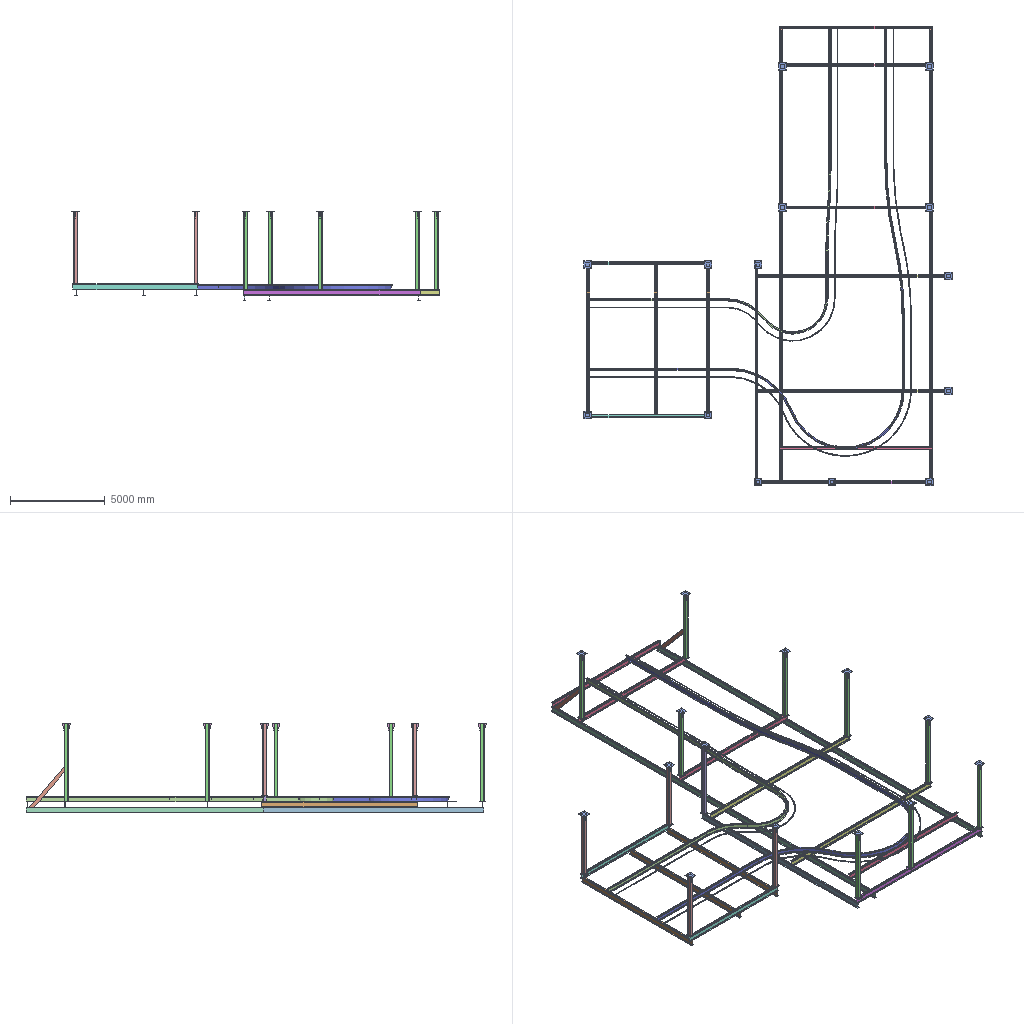Assembly | SolidWorks | 22 different items | 106 placed | box 19450 x 24300 x 4750 mm
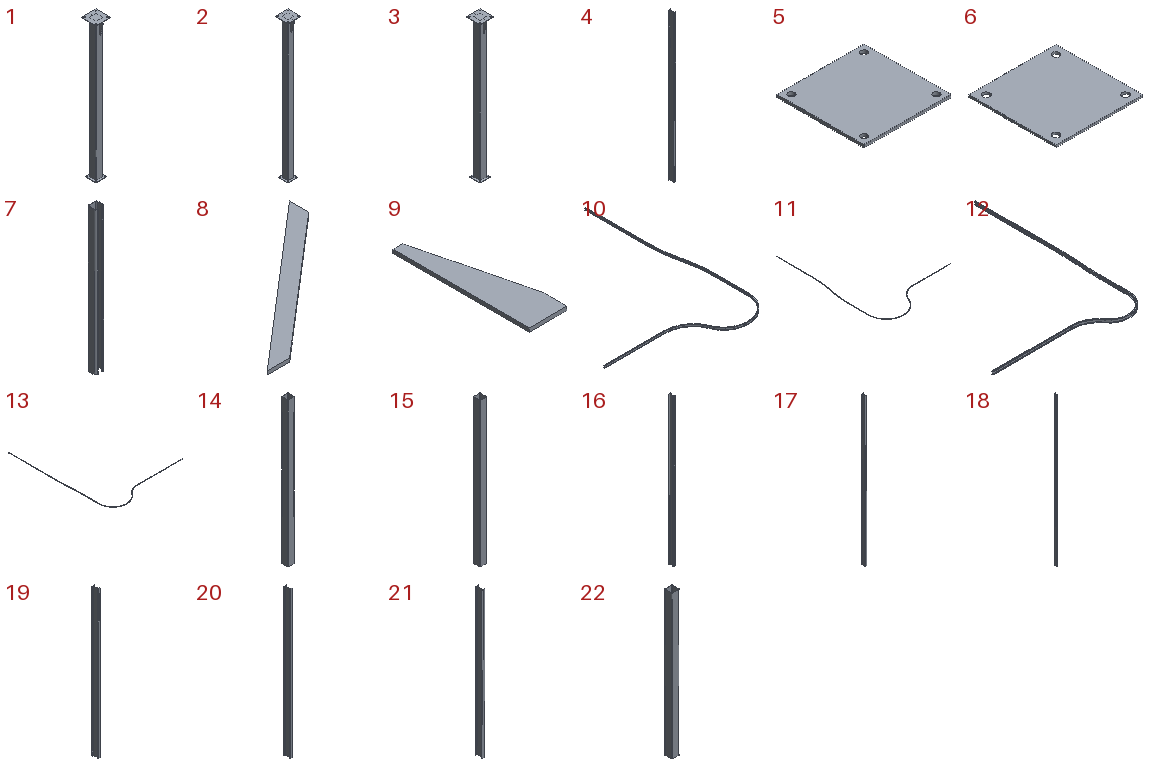Parts list (item | name | quantity | parent item | size | volume | features):
1 | (subassembly) | x4 | - | 400 x 400 x 3850 mm | 25640494 mm3 | -
2 | (subassembly) | x1 | - | 400 x 400 x 4450 mm | 29195042 mm3 | -
3 | (subassembly) | x9 | - | 400 x 400 x 4150 mm | 27417768 mm3 | -
4 | - | x1 | - | 150 x 300 x 9347 mm | 43725928 mm3 | features Extrusion 1
5 | - | x14 | in 1, 2, 3 | 300 x 300 x 10 mm | 884795 mm3 | features Extrusion 1
6 | - | x14 | in 1, 2, 3 | 400 x 400 x 10 mm | 1567830 mm3 | features Extrusion 1
7 | - | x1 | - | 32 x 30 x 500 mm | 85540 mm3 | features Extrusion 1
8 | - | x2 | - | 2174 x 1869 x 50 mm | 26646819 mm3 | features Extrusion 1
9 | - | x28 | in 1, 2, 3 | 100 x 360 x 10 mm | 249000 mm3 | features Extrusion 1
10 | - | x1 | - | 16778 x 22359 x 250 mm | 204415095 mm3 | features BaseBody 1
11 | - | x1 | - | 17149 x 22725 x 30 mm | 6973781 mm3 | features Sweep 1
12 | - | x1 | - | 12904 x 16279 x 250 mm | 148415394 mm3 | features BaseBody 1
13 | - | x1 | - | 13271 x 16645 x 30 mm | 5014402 mm3 | features Sweep 1
14 | - | x1 | in 2 | 200 x 200 x 4430 mm | 26244417 mm3 | features Extrusion 1
15 | - | x9 | in 3 | 200 x 200 x 4130 mm | 24467143 mm3 | features Extrusion 1
16 | - | x2 | - | 150 x 300 x 10347 mm | 48403999 mm3 | features Extrusion 1
17 | - | x1 | - | 150 x 300 x 11647 mm | 54485491 mm3 | features Extrusion 1
18 | - | x2 | - | 150 x 300 x 24174 mm | 113087685 mm3 | features Extrusion 1
19 | - | x3 | - | 150 x 300 x 8240 mm | 38547304 mm3 | features Extrusion 1
20 | - | x4 | - | 150 x 300 x 8060 mm | 37705251 mm3 | features Extrusion 1
21 | - | x2 | - | 150 x 300 x 6592 mm | 30837843 mm3 | features Extrusion 1
22 | - | x4 | in 1 | 200 x 200 x 3830 mm | 22689869 mm3 | features Extrusion 1
Mates (type | each side: item.copy, entity, surface, feature):
In the top assembly
Coincident | 5.1 face plane Boss-Extrude1 | 5.2 face plane Boss-Extrude1 | 2 times
Coincident | 5.1 face plane Boss-Extrude1 | 5.3 face plane Boss-Extrude1 | 2 times
Coincident | 5.1 face plane Boss-Extrude1 | 5.4 face plane Boss-Extrude1
Coincident | 5.2 face plane Boss-Extrude1 | 5.4 face plane Boss-Extrude1
Coincident | 5.3 face plane Boss-Extrude1 | 5.4 face plane Boss-Extrude1
Coincident | 5.1 face plane Boss-Extrude1 | 21.1 face plane Boss-Extrude1 | 2 times
Coincident | 21.1 face plane Boss-Extrude1 | 21.2 face plane Boss-Extrude1 | 2 times
Coincident | 5.2 face plane Boss-Extrude1 | 21.2 face plane Boss-Extrude1 | 2 times
DistanceDim | 22.1 face plane Boss-Extrude1 | 22.2 face plane Boss-Extrude1
Coincident | 19.1 face plane Boss-Extrude1 | 19.2 face plane Boss-Extrude1 | 2 times
Coincident | 19.1 face plane Boss-Extrude1 | 19.3 face plane Boss-Extrude1 | 2 times
Coincident | 21.1 face plane Boss-Extrude1 | 19.1 face plane Boss-Extrude1 | 2 times
DistanceDim | 21.1 face plane Boss-Extrude1 | 19.1 face plane Boss-Extrude1
Coincident | 21.1 face plane Boss-Extrude1 | 19.3 face plane Boss-Extrude1
DistanceDim | 19.2 face plane Boss-Extrude1 | 19.1 face plane Boss-Extrude1
Coincident | 5.5 face plane Boss-Extrude1 | 5.6 face plane Boss-Extrude1
Coincident | 5.3 face plane Boss-Extrude1 | 5.5 face plane Boss-Extrude1
DistanceDim | 22.3 face plane Boss-Extrude1 | 14.1 face plane Boss-Extrude1
DistanceDim | 14.1 face plane Boss-Extrude1 | 15.1 face plane Boss-Extrude1
Coincident | 5.7 face plane Boss-Extrude1 | 5.8 face plane Boss-Extrude1
Coincident | 5.7 face plane Boss-Extrude1 | 5.9 face plane Boss-Extrude1
Coincident | 5.7 face plane Boss-Extrude1 | 5.10 face plane Boss-Extrude1
Coincident | 5.7 face plane Boss-Extrude1 | 5.11 face plane Boss-Extrude1
Coincident | 5.7 face plane Boss-Extrude1 | 5.12 face plane Boss-Extrude1
Coincident | 5.7 face plane Boss-Extrude1 | 5.13 face plane Boss-Extrude1 | 2 times
Coincident | 5.7 face plane Boss-Extrude1 | 5.14 face plane Boss-Extrude1
Coincident | 5.6 face plane Boss-Extrude1 | 5.10 face plane Boss-Extrude1
Coincident | 5.10 face plane Boss-Extrude1 | 5.11 face plane Boss-Extrude1
Coincident | 5.11 face plane Boss-Extrude1 | 5.12 face plane Boss-Extrude1
Coincident | 5.12 face plane Boss-Extrude1 | 5.13 face plane Boss-Extrude1
Coincident | 5.9 face plane Boss-Extrude1 | 5.12 face plane Boss-Extrude1
Coincident | 5.8 face plane Boss-Extrude1 | 5.14 face plane Boss-Extrude1
DistanceDim | 22.3 face plane Boss-Extrude1 | 15.2 face plane Boss-Extrude1 | 2 times
Coincident | 15.2 face plane Boss-Extrude1 | 15.3 face plane Boss-Extrude1
DistanceDim | 15.2 face plane Boss-Extrude1 | 15.4 face plane Boss-Extrude1
DistanceDim | 15.5 face plane Boss-Extrude1 | 15.4 face plane Boss-Extrude1
DistanceDim | 15.6 face plane Boss-Extrude1 | 15.5 face plane Boss-Extrude1
DistanceDim | 15.7 face plane Boss-Extrude1 | 15.8 face plane Boss-Extrude1
Coincident | 20.1 face plane Boss-Extrude1 | 20.2 face plane Boss-Extrude1 | 2 times
Coincident | 5.13 face plane Boss-Extrude1 | 20.1 face plane Boss-Extrude1 | 2 times
Coincident | 6.1 face plane Boss-Extrude1 | 6.2 face plane Boss-Extrude1
Coincident | 5.5 face plane Boss-Extrude1 | 17.1 face plane Boss-Extrude1 | 2 times
Coincident | 16.1 face plane Boss-Extrude1 | 16.2 face plane Boss-Extrude1 | 2 times
Coincident | 5.8 face plane Boss-Extrude1 | 16.2 face plane Boss-Extrude1 | 2 times
Coincident | 5.11 face plane Boss-Extrude1 | 4.1 face plane Boss-Extrude1 | 2 times
Coincident | 18.1 face plane Boss-Extrude1 | 18.2 face plane Boss-Extrude1 | 2 times
Coincident | 20.1 face plane Boss-Extrude1 | 18.1 face plane Boss-Extrude1 | 3 times
Coincident | 20.1 face plane Boss-Extrude1 | 18.2 face plane Boss-Extrude1
Coincident | 16.2 face plane Boss-Extrude1 | 20.3 face plane Boss-Extrude1
Coincident | 4.1 face plane Boss-Extrude1 | 20.3 face plane Boss-Extrude1
Coincident | 6.2 face plane Boss-Extrude1 | 6.3 face plane Boss-Extrude1
Coincident | 4.1 face plane Boss-Extrude1 | 18.1 face plane Boss-Extrude1
DistanceDim | 5.3 face plane Boss-Extrude1 | 5.1 face plane Boss-Extrude1
Coincident | 6.4 face plane Boss-Extrude1 | 6.5 face plane Boss-Extrude1
Coincident | 20.1 face plane Boss-Extrude1 | 20.4 face plane Boss-Extrude1 | 2 times
Coincident | 5.7 face plane Boss-Extrude1 | 20.4 face plane Boss-Extrude1
Coincident | 15.2 face plane Boss-Extrude1 | 8.1 face plane Boss-Extrude1 | 2 times
Coincident | 18.1 face plane Boss-Extrude1 | 8.1 face plane Boss-Extrude1
Coincident | 15.4 face plane Boss-Extrude1 | 8.2 face plane Boss-Extrude1 | 2 times
Coincident | 18.2 face plane Boss-Extrude1 | 8.2 face plane Boss-Extrude1
DistanceDim | 16.2 face plane Boss-Extrude1 | 4.1 face plane Boss-Extrude1
DistanceDim | 16.1 face plane Boss-Extrude1 | 4.1 face plane Boss-Extrude1
DistanceDim | 15.9 face plane Boss-Extrude1 | 15.8 face plane Boss-Extrude1
DistanceDim | 15.6 face plane Boss-Extrude1 | 15.8 face plane Boss-Extrude1
Coincident | 19.1 face plane Boss-Extrude1 | 12.1 face plane Input 1 | 2 times
Coincident | 19.1 face plane Boss-Extrude1 | 10.1 face plane Input 1 | 2 times
Coincident | 20.1 face plane Boss-Extrude1 | 12.1 face plane Input 1
Coincident | 20.1 face plane Boss-Extrude1 | 10.1 face plane Input 1
Coincident | 19.1 face plane Boss-Extrude1 | 11.1 face plane Sweep1 | 2 times
Coincident | 20.1 face plane Boss-Extrude1 | 11.1 vertex
DistanceDim | 4.1 face plane Boss-Extrude1 | 5.11 face plane Boss-Extrude1
Coincident | 19.1 face plane Boss-Extrude1 | 13.1 face plane Sweep1 | 2 times
Coincident | 20.1 face plane Boss-Extrude1 | 13.1 vertex
In subassembly 3
Coincident | 15.10 face plane Boss-Extrude1 | 6.6 face plane Boss-Extrude1
DistanceDim | 15.10 face plane Boss-Extrude1 | 6.6 face plane Boss-Extrude1 | 2 times
Coincident | 15.10 face plane Boss-Extrude1 | 5.15 face plane Boss-Extrude1
DistanceDim | 5.15 face plane Boss-Extrude1 | 15.10 face plane Boss-Extrude1 | 2 times
Coincident | 6.6 face plane Boss-Extrude1 | 9.1 face plane Boss-Extrude1
Coincident | 15.10 face plane Boss-Extrude1 | 9.1 face plane Boss-Extrude1
DistanceDim | 9.1 face plane Boss-Extrude1 | 6.6 face plane Boss-Extrude1
Coincident | 6.6 face plane Boss-Extrude1 | 9.2 face plane Boss-Extrude1
Coincident | 9.1 face plane Boss-Extrude1 | 9.2 face plane Boss-Extrude1
Coincident | 15.10 face plane Boss-Extrude1 | 9.2 face plane Boss-Extrude1
In subassembly 1
Coincident | 22.4 face plane Boss-Extrude1 | 6.6 face plane Boss-Extrude1
DistanceDim | 22.4 face plane Boss-Extrude1 | 6.6 face plane Boss-Extrude1 | 2 times
Coincident | 22.4 face plane Boss-Extrude1 | 5.15 face plane Boss-Extrude1
DistanceDim | 5.15 face plane Boss-Extrude1 | 22.4 face plane Boss-Extrude1 | 2 times
Coincident | 6.6 face plane Boss-Extrude1 | 9.1 face plane Boss-Extrude1
Coincident | 22.4 face plane Boss-Extrude1 | 9.1 face plane Boss-Extrude1
DistanceDim | 9.1 face plane Boss-Extrude1 | 6.6 face plane Boss-Extrude1
Coincident | 6.6 face plane Boss-Extrude1 | 9.2 face plane Boss-Extrude1
Coincident | 9.1 face plane Boss-Extrude1 | 9.2 face plane Boss-Extrude1
Coincident | 22.4 face plane Boss-Extrude1 | 9.2 face plane Boss-Extrude1
In subassembly 2
Coincident | 14.2 face plane Boss-Extrude1 | 6.6 face plane Boss-Extrude1
DistanceDim | 14.2 face plane Boss-Extrude1 | 6.6 face plane Boss-Extrude1 | 2 times
Coincident | 14.2 face plane Boss-Extrude1 | 5.15 face plane Boss-Extrude1
DistanceDim | 5.15 face plane Boss-Extrude1 | 14.2 face plane Boss-Extrude1 | 2 times
Coincident | 6.6 face plane Boss-Extrude1 | 9.1 face plane Boss-Extrude1
Coincident | 14.2 face plane Boss-Extrude1 | 9.1 face plane Boss-Extrude1
DistanceDim | 9.1 face plane Boss-Extrude1 | 6.6 face plane Boss-Extrude1
Coincident | 6.6 face plane Boss-Extrude1 | 9.2 face plane Boss-Extrude1
Coincident | 9.1 face plane Boss-Extrude1 | 9.2 face plane Boss-Extrude1
Coincident | 14.2 face plane Boss-Extrude1 | 9.2 face plane Boss-Extrude1